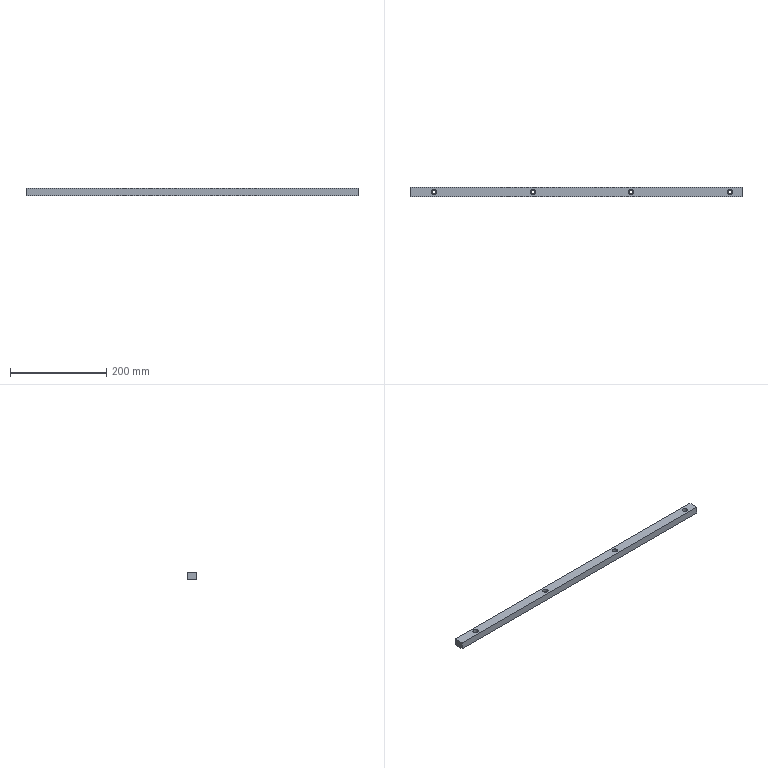Part | SolidWorks | features Extrusion 1, HoleWzd 1, ICE 1 | 1 solid | 26 faces | box 690 x 20 x 15 mm | volume 203293 mm3 | cylinder 16 | plane 10 | commonest cylinder face diameters 6.6 x8 11 x8
STEP:
#1=CARTESIAN_POINT('',(-313.,0.,8.2));
#2=VERTEX_POINT('',#1);
#3=CARTESIAN_POINT('',(-302.,0.,8.2));
#4=VERTEX_POINT('',#3);
#5=CARTESIAN_POINT('',(-307.5,0.,8.2));
#6=DIRECTION('',(0.,0.,1.));
#7=DIRECTION('',(1.,0.,0.));
#8=AXIS2_PLACEMENT_3D('',#5,#6,#7);
#9=CIRCLE('',#8,5.5);
#10=EDGE_CURVE('',#2,#4,#9,.T.);
#11=ORIENTED_EDGE('',*,*,#10,.F.);
#12=CARTESIAN_POINT('',(-313.,0.,15.));
#13=VERTEX_POINT('',#12);
#14=CARTESIAN_POINT('',(-313.,0.,15.));
#15=DIRECTION('',(0.,0.,1.));
#16=VECTOR('',#15,1000.);
#17=LINE('',#14,#16);
#18=EDGE_CURVE('',#2,#13,#17,.T.);
#19=ORIENTED_EDGE('',*,*,#18,.T.);
#20=CARTESIAN_POINT('',(-302.,0.,15.));
#21=VERTEX_POINT('',#20);
#22=CARTESIAN_POINT('',(-307.5,0.,15.));
#23=DIRECTION('',(0.,0.,1.));
#24=DIRECTION('',(1.,0.,0.));
#25=AXIS2_PLACEMENT_3D('',#22,#23,#24);
#26=CIRCLE('',#25,5.5);
#27=EDGE_CURVE('',#13,#21,#26,.T.);
#28=ORIENTED_EDGE('',*,*,#27,.T.);
#29=CARTESIAN_POINT('',(-302.,0.,15.));
#30=DIRECTION('',(0.,0.,1.));
#31=VECTOR('',#30,1000.);
#32=LINE('',#29,#31);
#33=EDGE_CURVE('',#4,#21,#32,.T.);
#34=ORIENTED_EDGE('',*,*,#33,.F.);
#35=EDGE_LOOP('',(#11,#19,#28,#34));
#36=FACE_OUTER_BOUND('',#35,.T.);
#37=CARTESIAN_POINT('',(-307.5,0.,15.));
#38=DIRECTION('',(0.,0.,1.));
#39=DIRECTION('',(1.,0.,0.));
#40=AXIS2_PLACEMENT_3D('',#37,#38,#39);
#41=CYLINDRICAL_SURFACE('',#40,5.5);
#42=ADVANCED_FACE('',(#36),#41,.F.);
#43=CARTESIAN_POINT('',(-310.8,0.,0.));
#44=VERTEX_POINT('',#43);
#45=CARTESIAN_POINT('',(-304.2,0.,0.));
#46=VERTEX_POINT('',#45);
#47=CARTESIAN_POINT('',(-307.5,0.,0.));
#48=DIRECTION('',(0.,0.,1.));
#49=DIRECTION('',(1.,0.,0.));
#50=AXIS2_PLACEMENT_3D('',#47,#48,#49);
#51=CIRCLE('',#50,3.3);
#52=EDGE_CURVE('',#44,#46,#51,.T.);
#53=ORIENTED_EDGE('',*,*,#52,.F.);
#54=CARTESIAN_POINT('',(-310.8,0.,8.2));
#55=VERTEX_POINT('',#54);
#56=CARTESIAN_POINT('',(-310.8,0.,15.));
#57=DIRECTION('',(0.,0.,1.));
#58=VECTOR('',#57,1000.);
#59=LINE('',#56,#58);
#60=EDGE_CURVE('',#44,#55,#59,.T.);
#61=ORIENTED_EDGE('',*,*,#60,.T.);
#62=CARTESIAN_POINT('',(-304.2,0.,8.2));
#63=VERTEX_POINT('',#62);
#64=CARTESIAN_POINT('',(-307.5,0.,8.2));
#65=DIRECTION('',(0.,0.,1.));
#66=DIRECTION('',(1.,0.,0.));
#67=AXIS2_PLACEMENT_3D('',#64,#65,#66);
#68=CIRCLE('',#67,3.3);
#69=EDGE_CURVE('',#55,#63,#68,.T.);
#70=ORIENTED_EDGE('',*,*,#69,.T.);
#71=CARTESIAN_POINT('',(-304.2,0.,15.));
#72=DIRECTION('',(0.,0.,1.));
#73=VECTOR('',#72,1000.);
#74=LINE('',#71,#73);
#75=EDGE_CURVE('',#46,#63,#74,.T.);
#76=ORIENTED_EDGE('',*,*,#75,.F.);
#77=EDGE_LOOP('',(#53,#61,#70,#76));
#78=FACE_OUTER_BOUND('',#77,.T.);
#79=CARTESIAN_POINT('',(-307.5,0.,15.));
#80=DIRECTION('',(0.,0.,1.));
#81=DIRECTION('',(1.,0.,0.));
#82=AXIS2_PLACEMENT_3D('',#79,#80,#81);
#83=CYLINDRICAL_SURFACE('',#82,3.3);
#84=ADVANCED_FACE('',(#78),#83,.F.);
#85=CARTESIAN_POINT('',(302.,0.,8.2));
#86=VERTEX_POINT('',#85);
#87=CARTESIAN_POINT('',(313.,0.,8.2));
#88=VERTEX_POINT('',#87);
#89=CARTESIAN_POINT('',(307.5,0.,8.2));
#90=DIRECTION('',(0.,0.,1.));
#91=DIRECTION('',(1.,0.,0.));
#92=AXIS2_PLACEMENT_3D('',#89,#90,#91);
#93=CIRCLE('',#92,5.5);
#94=EDGE_CURVE('',#86,#88,#93,.T.);
#95=ORIENTED_EDGE('',*,*,#94,.F.);
#96=CARTESIAN_POINT('',(302.,0.,15.));
#97=VERTEX_POINT('',#96);
#98=CARTESIAN_POINT('',(302.,0.,15.));
#99=DIRECTION('',(0.,0.,1.));
#100=VECTOR('',#99,1000.);
#101=LINE('',#98,#100);
#102=EDGE_CURVE('',#86,#97,#101,.T.);
#103=ORIENTED_EDGE('',*,*,#102,.T.);
#104=CARTESIAN_POINT('',(313.,0.,15.));
#105=VERTEX_POINT('',#104);
#106=CARTESIAN_POINT('',(307.5,0.,15.));
#107=DIRECTION('',(0.,0.,1.));
#108=DIRECTION('',(1.,0.,0.));
#109=AXIS2_PLACEMENT_3D('',#106,#107,#108);
#110=CIRCLE('',#109,5.5);
#111=EDGE_CURVE('',#97,#105,#110,.T.);
#112=ORIENTED_EDGE('',*,*,#111,.T.);
#113=CARTESIAN_POINT('',(313.,0.,15.));
#114=DIRECTION('',(0.,0.,1.));
#115=VECTOR('',#114,1000.);
#116=LINE('',#113,#115);
#117=EDGE_CURVE('',#88,#105,#116,.T.);
#118=ORIENTED_EDGE('',*,*,#117,.F.);
#119=EDGE_LOOP('',(#95,#103,#112,#118));
#120=FACE_OUTER_BOUND('',#119,.T.);
#121=CARTESIAN_POINT('',(307.5,0.,15.));
#122=DIRECTION('',(0.,0.,1.));
#123=DIRECTION('',(1.,0.,0.));
#124=AXIS2_PLACEMENT_3D('',#121,#122,#123);
#125=CYLINDRICAL_SURFACE('',#124,5.5);
#126=ADVANCED_FACE('',(#120),#125,.F.);
#127=CARTESIAN_POINT('',(304.2,0.,0.));
#128=VERTEX_POINT('',#127);
#129=CARTESIAN_POINT('',(310.8,0.,0.));
#130=VERTEX_POINT('',#129);
#131=CARTESIAN_POINT('',(307.5,0.,0.));
#132=DIRECTION('',(0.,0.,1.));
#133=DIRECTION('',(1.,0.,0.));
#134=AXIS2_PLACEMENT_3D('',#131,#132,#133);
#135=CIRCLE('',#134,3.3);
#136=EDGE_CURVE('',#128,#130,#135,.T.);
#137=ORIENTED_EDGE('',*,*,#136,.F.);
#138=CARTESIAN_POINT('',(304.2,0.,8.2));
#139=VERTEX_POINT('',#138);
#140=CARTESIAN_POINT('',(304.2,0.,15.));
#141=DIRECTION('',(0.,0.,1.));
#142=VECTOR('',#141,1000.);
#143=LINE('',#140,#142);
#144=EDGE_CURVE('',#128,#139,#143,.T.);
#145=ORIENTED_EDGE('',*,*,#144,.T.);
#146=CARTESIAN_POINT('',(310.8,0.,8.2));
#147=VERTEX_POINT('',#146);
#148=CARTESIAN_POINT('',(307.5,0.,8.2));
#149=DIRECTION('',(0.,0.,1.));
#150=DIRECTION('',(1.,0.,0.));
#151=AXIS2_PLACEMENT_3D('',#148,#149,#150);
#152=CIRCLE('',#151,3.3);
#153=EDGE_CURVE('',#139,#147,#152,.T.);
#154=ORIENTED_EDGE('',*,*,#153,.T.);
#155=CARTESIAN_POINT('',(310.8,0.,15.));
#156=DIRECTION('',(0.,0.,1.));
#157=VECTOR('',#156,1000.);
#158=LINE('',#155,#157);
#159=EDGE_CURVE('',#130,#147,#158,.T.);
#160=ORIENTED_EDGE('',*,*,#159,.F.);
#161=EDGE_LOOP('',(#137,#145,#154,#160));
#162=FACE_OUTER_BOUND('',#161,.T.);
#163=CARTESIAN_POINT('',(307.5,0.,15.));
#164=DIRECTION('',(0.,0.,1.));
#165=DIRECTION('',(1.,0.,0.));
#166=AXIS2_PLACEMENT_3D('',#163,#164,#165);
#167=CYLINDRICAL_SURFACE('',#166,3.3);
#168=ADVANCED_FACE('',(#162),#167,.F.);
#169=CARTESIAN_POINT('',(-108.,0.,8.2));
#170=VERTEX_POINT('',#169);
#171=CARTESIAN_POINT('',(-97.,0.,8.2));
#172=VERTEX_POINT('',#171);
#173=CARTESIAN_POINT('',(-102.5,0.,8.2));
#174=DIRECTION('',(0.,0.,1.));
#175=DIRECTION('',(1.,0.,0.));
#176=AXIS2_PLACEMENT_3D('',#173,#174,#175);
#177=CIRCLE('',#176,5.5);
#178=EDGE_CURVE('',#170,#172,#177,.T.);
#179=ORIENTED_EDGE('',*,*,#178,.F.);
#180=CARTESIAN_POINT('',(-108.,0.,15.));
#181=VERTEX_POINT('',#180);
#182=CARTESIAN_POINT('',(-108.,0.,15.));
#183=DIRECTION('',(0.,0.,1.));
#184=VECTOR('',#183,1000.);
#185=LINE('',#182,#184);
#186=EDGE_CURVE('',#170,#181,#185,.T.);
#187=ORIENTED_EDGE('',*,*,#186,.T.);
#188=CARTESIAN_POINT('',(-97.,0.,15.));
#189=VERTEX_POINT('',#188);
#190=CARTESIAN_POINT('',(-102.5,0.,15.));
#191=DIRECTION('',(0.,0.,1.));
#192=DIRECTION('',(1.,0.,0.));
#193=AXIS2_PLACEMENT_3D('',#190,#191,#192);
#194=CIRCLE('',#193,5.5);
#195=EDGE_CURVE('',#181,#189,#194,.T.);
#196=ORIENTED_EDGE('',*,*,#195,.T.);
#197=CARTESIAN_POINT('',(-97.,0.,15.));
#198=DIRECTION('',(0.,0.,1.));
#199=VECTOR('',#198,1000.);
#200=LINE('',#197,#199);
#201=EDGE_CURVE('',#172,#189,#200,.T.);
#202=ORIENTED_EDGE('',*,*,#201,.F.);
#203=EDGE_LOOP('',(#179,#187,#196,#202));
#204=FACE_OUTER_BOUND('',#203,.T.);
#205=CARTESIAN_POINT('',(-102.5,0.,15.));
#206=DIRECTION('',(0.,0.,1.));
#207=DIRECTION('',(1.,0.,0.));
#208=AXIS2_PLACEMENT_3D('',#205,#206,#207);
#209=CYLINDRICAL_SURFACE('',#208,5.5);
#210=ADVANCED_FACE('',(#204),#209,.F.);
#211=CARTESIAN_POINT('',(-105.8,0.,0.));
#212=VERTEX_POINT('',#211);
#213=CARTESIAN_POINT('',(-99.2,0.,0.));
#214=VERTEX_POINT('',#213);
#215=CARTESIAN_POINT('',(-102.5,0.,0.));
#216=DIRECTION('',(0.,0.,1.));
#217=DIRECTION('',(1.,0.,0.));
#218=AXIS2_PLACEMENT_3D('',#215,#216,#217);
#219=CIRCLE('',#218,3.3);
#220=EDGE_CURVE('',#212,#214,#219,.T.);
#221=ORIENTED_EDGE('',*,*,#220,.F.);
#222=CARTESIAN_POINT('',(-105.8,0.,8.2));
#223=VERTEX_POINT('',#222);
#224=CARTESIAN_POINT('',(-105.8,0.,15.));
#225=DIRECTION('',(0.,0.,1.));
#226=VECTOR('',#225,1000.);
#227=LINE('',#224,#226);
#228=EDGE_CURVE('',#212,#223,#227,.T.);
#229=ORIENTED_EDGE('',*,*,#228,.T.);
#230=CARTESIAN_POINT('',(-99.2,0.,8.2));
#231=VERTEX_POINT('',#230);
#232=CARTESIAN_POINT('',(-102.5,0.,8.2));
#233=DIRECTION('',(0.,0.,1.));
#234=DIRECTION('',(1.,0.,0.));
#235=AXIS2_PLACEMENT_3D('',#232,#233,#234);
#236=CIRCLE('',#235,3.3);
#237=EDGE_CURVE('',#223,#231,#236,.T.);
#238=ORIENTED_EDGE('',*,*,#237,.T.);
#239=CARTESIAN_POINT('',(-99.2,0.,15.));
#240=DIRECTION('',(0.,0.,1.));
#241=VECTOR('',#240,1000.);
#242=LINE('',#239,#241);
#243=EDGE_CURVE('',#214,#231,#242,.T.);
#244=ORIENTED_EDGE('',*,*,#243,.F.);
#245=EDGE_LOOP('',(#221,#229,#238,#244));
#246=FACE_OUTER_BOUND('',#245,.T.);
#247=CARTESIAN_POINT('',(-102.5,0.,15.));
#248=DIRECTION('',(0.,0.,1.));
#249=DIRECTION('',(1.,0.,0.));
#250=AXIS2_PLACEMENT_3D('',#247,#248,#249);
#251=CYLINDRICAL_SURFACE('',#250,3.3);
#252=ADVANCED_FACE('',(#246),#251,.F.);
#253=CARTESIAN_POINT('',(97.,0.,8.2));
#254=VERTEX_POINT('',#253);
#255=CARTESIAN_POINT('',(108.,0.,8.2));
#256=VERTEX_POINT('',#255);
#257=CARTESIAN_POINT('',(102.5,0.,8.2));
#258=DIRECTION('',(0.,0.,1.));
#259=DIRECTION('',(1.,0.,0.));
#260=AXIS2_PLACEMENT_3D('',#257,#258,#259);
#261=CIRCLE('',#260,5.5);
#262=EDGE_CURVE('',#254,#256,#261,.T.);
#263=ORIENTED_EDGE('',*,*,#262,.F.);
#264=CARTESIAN_POINT('',(97.,0.,15.));
#265=VERTEX_POINT('',#264);
#266=CARTESIAN_POINT('',(97.,0.,15.));
#267=DIRECTION('',(0.,0.,1.));
#268=VECTOR('',#267,1000.);
#269=LINE('',#266,#268);
#270=EDGE_CURVE('',#254,#265,#269,.T.);
#271=ORIENTED_EDGE('',*,*,#270,.T.);
#272=CARTESIAN_POINT('',(108.,0.,15.));
#273=VERTEX_POINT('',#272);
#274=CARTESIAN_POINT('',(102.5,0.,15.));
#275=DIRECTION('',(0.,0.,1.));
#276=DIRECTION('',(1.,0.,0.));
#277=AXIS2_PLACEMENT_3D('',#274,#275,#276);
#278=CIRCLE('',#277,5.5);
#279=EDGE_CURVE('',#265,#273,#278,.T.);
#280=ORIENTED_EDGE('',*,*,#279,.T.);
#281=CARTESIAN_POINT('',(108.,0.,15.));
#282=DIRECTION('',(0.,0.,1.));
#283=VECTOR('',#282,1000.);
#284=LINE('',#281,#283);
#285=EDGE_CURVE('',#256,#273,#284,.T.);
#286=ORIENTED_EDGE('',*,*,#285,.F.);
#287=EDGE_LOOP('',(#263,#271,#280,#286));
#288=FACE_OUTER_BOUND('',#287,.T.);
#289=CARTESIAN_POINT('',(102.5,0.,15.));
#290=DIRECTION('',(0.,0.,1.));
#291=DIRECTION('',(1.,0.,0.));
#292=AXIS2_PLACEMENT_3D('',#289,#290,#291);
#293=CYLINDRICAL_SURFACE('',#292,5.5);
#294=ADVANCED_FACE('',(#288),#293,.F.);
#295=CARTESIAN_POINT('',(99.2,0.,0.));
#296=VERTEX_POINT('',#295);
#297=CARTESIAN_POINT('',(105.8,0.,0.));
#298=VERTEX_POINT('',#297);
#299=CARTESIAN_POINT('',(102.5,0.,0.));
#300=DIRECTION('',(0.,0.,1.));
#301=DIRECTION('',(1.,0.,0.));
#302=AXIS2_PLACEMENT_3D('',#299,#300,#301);
#303=CIRCLE('',#302,3.3);
#304=EDGE_CURVE('',#296,#298,#303,.T.);
#305=ORIENTED_EDGE('',*,*,#304,.F.);
#306=CARTESIAN_POINT('',(99.2,0.,8.2));
#307=VERTEX_POINT('',#306);
#308=CARTESIAN_POINT('',(99.2,0.,15.));
#309=DIRECTION('',(0.,0.,1.));
#310=VECTOR('',#309,1000.);
#311=LINE('',#308,#310);
#312=EDGE_CURVE('',#296,#307,#311,.T.);
#313=ORIENTED_EDGE('',*,*,#312,.T.);
#314=CARTESIAN_POINT('',(105.8,0.,8.2));
#315=VERTEX_POINT('',#314);
#316=CARTESIAN_POINT('',(102.5,0.,8.2));
#317=DIRECTION('',(0.,0.,1.));
#318=DIRECTION('',(1.,0.,0.));
#319=AXIS2_PLACEMENT_3D('',#316,#317,#318);
#320=CIRCLE('',#319,3.3);
#321=EDGE_CURVE('',#307,#315,#320,.T.);
#322=ORIENTED_EDGE('',*,*,#321,.T.);
#323=CARTESIAN_POINT('',(105.8,0.,15.));
#324=DIRECTION('',(0.,0.,1.));
#325=VECTOR('',#324,1000.);
#326=LINE('',#323,#325);
#327=EDGE_CURVE('',#298,#315,#326,.T.);
#328=ORIENTED_EDGE('',*,*,#327,.F.);
#329=EDGE_LOOP('',(#305,#313,#322,#328));
#330=FACE_OUTER_BOUND('',#329,.T.);
#331=CARTESIAN_POINT('',(102.5,0.,15.));
#332=DIRECTION('',(0.,0.,1.));
#333=DIRECTION('',(1.,0.,0.));
#334=AXIS2_PLACEMENT_3D('',#331,#332,#333);
#335=CYLINDRICAL_SURFACE('',#334,3.3);
#336=ADVANCED_FACE('',(#330),#335,.F.);
#337=CARTESIAN_POINT('',(332.5,-10.,0.));
#338=VERTEX_POINT('',#337);
#339=CARTESIAN_POINT('',(332.5,10.,0.));
#340=VERTEX_POINT('',#339);
#341=CARTESIAN_POINT('',(332.5,10.,0.));
#342=DIRECTION('',(0.,1.,0.));
#343=VECTOR('',#342,1000.);
#344=LINE('',#341,#343);
#345=EDGE_CURVE('',#338,#340,#344,.T.);
#346=ORIENTED_EDGE('',*,*,#345,.T.);
#347=CARTESIAN_POINT('',(332.5,10.,15.));
#348=VERTEX_POINT('',#347);
#349=CARTESIAN_POINT('',(332.5,10.,15.));
#350=DIRECTION('',(0.,0.,-1.));
#351=VECTOR('',#350,1000.);
#352=LINE('',#349,#351);
#353=EDGE_CURVE('',#348,#340,#352,.T.);
#354=ORIENTED_EDGE('',*,*,#353,.F.);
#355=CARTESIAN_POINT('',(332.5,-10.,15.));
#356=VERTEX_POINT('',#355);
#357=CARTESIAN_POINT('',(332.5,10.,15.));
#358=DIRECTION('',(0.,1.,0.));
#359=VECTOR('',#358,1000.);
#360=LINE('',#357,#359);
#361=EDGE_CURVE('',#356,#348,#360,.T.);
#362=ORIENTED_EDGE('',*,*,#361,.F.);
#363=CARTESIAN_POINT('',(332.5,-10.,15.));
#364=DIRECTION('',(0.,0.,-1.));
#365=VECTOR('',#364,1000.);
#366=LINE('',#363,#365);
#367=EDGE_CURVE('',#356,#338,#366,.T.);
#368=ORIENTED_EDGE('',*,*,#367,.T.);
#369=EDGE_LOOP('',(#346,#354,#362,#368));
#370=FACE_OUTER_BOUND('',#369,.T.);
#371=CARTESIAN_POINT('',(332.5,10.,15.));
#372=DIRECTION('',(-1.,0.,0.));
#373=DIRECTION('',(0.,0.,1.));
#374=AXIS2_PLACEMENT_3D('',#371,#372,#373);
#375=PLANE('',#374);
#376=ADVANCED_FACE('',(#370),#375,.F.);
#377=CARTESIAN_POINT('',(-357.5,10.,0.));
#378=VERTEX_POINT('',#377);
#379=CARTESIAN_POINT('',(-332.5,10.,0.));
#380=DIRECTION('',(-1.,0.,0.));
#381=VECTOR('',#380,1000.);
#382=LINE('',#379,#381);
#383=EDGE_CURVE('',#340,#378,#382,.T.);
#384=ORIENTED_EDGE('',*,*,#383,.T.);
#385=CARTESIAN_POINT('',(-357.5,10.,15.));
#386=VERTEX_POINT('',#385);
#387=CARTESIAN_POINT('',(-357.5,10.,15.));
#388=DIRECTION('',(0.,0.,-1.));
#389=VECTOR('',#388,1000.);
#390=LINE('',#387,#389);
#391=EDGE_CURVE('',#386,#378,#390,.T.);
#392=ORIENTED_EDGE('',*,*,#391,.F.);
#393=CARTESIAN_POINT('',(-332.5,10.,15.));
#394=DIRECTION('',(-1.,0.,0.));
#395=VECTOR('',#394,1000.);
#396=LINE('',#393,#395);
#397=EDGE_CURVE('',#348,#386,#396,.T.);
#398=ORIENTED_EDGE('',*,*,#397,.F.);
#399=ORIENTED_EDGE('',*,*,#353,.T.);
#400=EDGE_LOOP('',(#384,#392,#398,#399));
#401=FACE_OUTER_BOUND('',#400,.T.);
#402=CARTESIAN_POINT('',(-332.5,10.,15.));
#403=DIRECTION('',(0.,-1.,0.));
#404=DIRECTION('',(0.,0.,-1.));
#405=AXIS2_PLACEMENT_3D('',#402,#403,#404);
#406=PLANE('',#405);
#407=ADVANCED_FACE('',(#401),#406,.F.);
#408=CARTESIAN_POINT('',(-357.5,-10.,0.));
#409=VERTEX_POINT('',#408);
#410=CARTESIAN_POINT('',(-332.5,-10.,0.));
#411=DIRECTION('',(1.,0.,0.));
#412=VECTOR('',#411,1000.);
#413=LINE('',#410,#412);
#414=EDGE_CURVE('',#409,#338,#413,.T.);
#415=ORIENTED_EDGE('',*,*,#414,.T.);
#416=ORIENTED_EDGE('',*,*,#367,.F.);
#417=CARTESIAN_POINT('',(-357.5,-10.,15.));
#418=VERTEX_POINT('',#417);
#419=CARTESIAN_POINT('',(-332.5,-10.,15.));
#420=DIRECTION('',(1.,0.,0.));
#421=VECTOR('',#420,1000.);
#422=LINE('',#419,#421);
#423=EDGE_CURVE('',#418,#356,#422,.T.);
#424=ORIENTED_EDGE('',*,*,#423,.F.);
#425=CARTESIAN_POINT('',(-357.5,-10.,0.));
#426=DIRECTION('',(0.,0.,1.));
#427=VECTOR('',#426,1000.);
#428=LINE('',#425,#427);
#429=EDGE_CURVE('',#409,#418,#428,.T.);
#430=ORIENTED_EDGE('',*,*,#429,.F.);
#431=EDGE_LOOP('',(#415,#416,#424,#430));
#432=FACE_OUTER_BOUND('',#431,.T.);
#433=CARTESIAN_POINT('',(-332.5,-10.,15.));
#434=DIRECTION('',(0.,1.,0.));
#435=DIRECTION('',(0.,0.,1.));
#436=AXIS2_PLACEMENT_3D('',#433,#434,#435);
#437=PLANE('',#436);
#438=ADVANCED_FACE('',(#432),#437,.F.);
#439=CARTESIAN_POINT('',(-307.5,0.,15.));
#440=DIRECTION('',(0.,0.,1.));
#441=DIRECTION('',(1.,0.,0.));
#442=AXIS2_PLACEMENT_3D('',#439,#440,#441);
#443=CIRCLE('',#442,5.5);
#444=EDGE_CURVE('',#21,#13,#443,.T.);
#445=ORIENTED_EDGE('',*,*,#444,.F.);
#446=ORIENTED_EDGE('',*,*,#27,.F.);
#447=EDGE_LOOP('',(#445,#446));
#448=FACE_BOUND('',#447,.T.);
#449=CARTESIAN_POINT('',(307.5,0.,15.));
#450=DIRECTION('',(0.,0.,1.));
#451=DIRECTION('',(1.,0.,0.));
#452=AXIS2_PLACEMENT_3D('',#449,#450,#451);
#453=CIRCLE('',#452,5.5);
#454=EDGE_CURVE('',#105,#97,#453,.T.);
#455=ORIENTED_EDGE('',*,*,#454,.F.);
#456=ORIENTED_EDGE('',*,*,#111,.F.);
#457=EDGE_LOOP('',(#455,#456));
#458=FACE_BOUND('',#457,.T.);
#459=CARTESIAN_POINT('',(-102.5,0.,15.));
#460=DIRECTION('',(0.,0.,1.));
#461=DIRECTION('',(1.,0.,0.));
#462=AXIS2_PLACEMENT_3D('',#459,#460,#461);
#463=CIRCLE('',#462,5.5);
#464=EDGE_CURVE('',#189,#181,#463,.T.);
#465=ORIENTED_EDGE('',*,*,#464,.F.);
#466=ORIENTED_EDGE('',*,*,#195,.F.);
#467=EDGE_LOOP('',(#465,#466));
#468=FACE_BOUND('',#467,.T.);
#469=CARTESIAN_POINT('',(102.5,0.,15.));
#470=DIRECTION('',(0.,0.,1.));
#471=DIRECTION('',(1.,0.,0.));
#472=AXIS2_PLACEMENT_3D('',#469,#470,#471);
#473=CIRCLE('',#472,5.5);
#474=EDGE_CURVE('',#273,#265,#473,.T.);
#475=ORIENTED_EDGE('',*,*,#474,.F.);
#476=ORIENTED_EDGE('',*,*,#279,.F.);
#477=EDGE_LOOP('',(#475,#476));
#478=FACE_BOUND('',#477,.T.);
#479=ORIENTED_EDGE('',*,*,#361,.T.);
#480=ORIENTED_EDGE('',*,*,#397,.T.);
#481=CARTESIAN_POINT('',(-357.5,-10.,15.));
#482=DIRECTION('',(0.,1.,0.));
#483=VECTOR('',#482,1000.);
#484=LINE('',#481,#483);
#485=EDGE_CURVE('',#418,#386,#484,.T.);
#486=ORIENTED_EDGE('',*,*,#485,.F.);
#487=ORIENTED_EDGE('',*,*,#423,.T.);
#488=EDGE_LOOP('',(#479,#480,#486,#487));
#489=FACE_OUTER_BOUND('',#488,.T.);
#490=CARTESIAN_POINT('',(0.,0.,15.));
#491=DIRECTION('',(0.,0.,1.));
#492=DIRECTION('',(1.,0.,0.));
#493=AXIS2_PLACEMENT_3D('',#490,#491,#492);
#494=PLANE('',#493);
#495=ADVANCED_FACE('',(#448,#458,#468,#478,#489),#494,.T.);
#496=CARTESIAN_POINT('',(-307.5,0.,0.));
#497=DIRECTION('',(0.,0.,1.));
#498=DIRECTION('',(1.,0.,0.));
#499=AXIS2_PLACEMENT_3D('',#496,#497,#498);
#500=CIRCLE('',#499,3.3);
#501=EDGE_CURVE('',#46,#44,#500,.T.);
#502=ORIENTED_EDGE('',*,*,#501,.T.);
#503=ORIENTED_EDGE('',*,*,#52,.T.);
#504=EDGE_LOOP('',(#502,#503));
#505=FACE_BOUND('',#504,.T.);
#506=CARTESIAN_POINT('',(307.5,0.,0.));
#507=DIRECTION('',(0.,0.,1.));
#508=DIRECTION('',(1.,0.,0.));
#509=AXIS2_PLACEMENT_3D('',#506,#507,#508);
#510=CIRCLE('',#509,3.3);
#511=EDGE_CURVE('',#130,#128,#510,.T.);
#512=ORIENTED_EDGE('',*,*,#511,.T.);
#513=ORIENTED_EDGE('',*,*,#136,.T.);
#514=EDGE_LOOP('',(#512,#513));
#515=FACE_BOUND('',#514,.T.);
#516=CARTESIAN_POINT('',(-102.5,0.,0.));
#517=DIRECTION('',(0.,0.,1.));
#518=DIRECTION('',(1.,0.,0.));
#519=AXIS2_PLACEMENT_3D('',#516,#517,#518);
#520=CIRCLE('',#519,3.3);
#521=EDGE_CURVE('',#214,#212,#520,.T.);
#522=ORIENTED_EDGE('',*,*,#521,.T.);
#523=ORIENTED_EDGE('',*,*,#220,.T.);
#524=EDGE_LOOP('',(#522,#523));
#525=FACE_BOUND('',#524,.T.);
#526=CARTESIAN_POINT('',(102.5,0.,0.));
#527=DIRECTION('',(0.,0.,1.));
#528=DIRECTION('',(1.,0.,0.));
#529=AXIS2_PLACEMENT_3D('',#526,#527,#528);
#530=CIRCLE('',#529,3.3);
#531=EDGE_CURVE('',#298,#296,#530,.T.);
#532=ORIENTED_EDGE('',*,*,#531,.T.);
#533=ORIENTED_EDGE('',*,*,#304,.T.);
#534=EDGE_LOOP('',(#532,#533));
#535=FACE_BOUND('',#534,.T.);
#536=ORIENTED_EDGE('',*,*,#345,.F.);
#537=ORIENTED_EDGE('',*,*,#414,.F.);
#538=CARTESIAN_POINT('',(-357.5,10.,0.));
#539=DIRECTION('',(0.,-1.,0.));
#540=VECTOR('',#539,1000.);
#541=LINE('',#538,#540);
#542=EDGE_CURVE('',#378,#409,#541,.T.);
#543=ORIENTED_EDGE('',*,*,#542,.F.);
#544=ORIENTED_EDGE('',*,*,#383,.F.);
#545=EDGE_LOOP('',(#536,#537,#543,#544));
#546=FACE_OUTER_BOUND('',#545,.T.);
#547=CARTESIAN_POINT('',(0.,0.,0.));
#548=DIRECTION('',(0.,0.,1.));
#549=DIRECTION('',(1.,0.,0.));
#550=AXIS2_PLACEMENT_3D('',#547,#548,#549);
#551=PLANE('',#550);
#552=ADVANCED_FACE('',(#505,#515,#525,#535,#546),#551,.F.);
#553=ORIENTED_EDGE('',*,*,#312,.F.);
#554=ORIENTED_EDGE('',*,*,#531,.F.);
#555=ORIENTED_EDGE('',*,*,#327,.T.);
#556=CARTESIAN_POINT('',(102.5,0.,8.2));
#557=DIRECTION('',(0.,0.,1.));
#558=DIRECTION('',(1.,0.,0.));
#559=AXIS2_PLACEMENT_3D('',#556,#557,#558);
#560=CIRCLE('',#559,3.3);
#561=EDGE_CURVE('',#315,#307,#560,.T.);
#562=ORIENTED_EDGE('',*,*,#561,.T.);
#563=EDGE_LOOP('',(#553,#554,#555,#562));
#564=FACE_OUTER_BOUND('',#563,.T.);
#565=CARTESIAN_POINT('',(102.5,0.,15.));
#566=DIRECTION('',(0.,0.,1.));
#567=DIRECTION('',(1.,0.,0.));
#568=AXIS2_PLACEMENT_3D('',#565,#566,#567);
#569=CYLINDRICAL_SURFACE('',#568,3.3);
#570=ADVANCED_FACE('',(#564),#569,.F.);
#571=ORIENTED_EDGE('',*,*,#561,.F.);
#572=ORIENTED_EDGE('',*,*,#321,.F.);
#573=EDGE_LOOP('',(#571,#572));
#574=FACE_BOUND('',#573,.T.);
#575=CARTESIAN_POINT('',(102.5,0.,8.2));
#576=DIRECTION('',(0.,0.,1.));
#577=DIRECTION('',(1.,0.,0.));
#578=AXIS2_PLACEMENT_3D('',#575,#576,#577);
#579=CIRCLE('',#578,5.5);
#580=EDGE_CURVE('',#256,#254,#579,.T.);
#581=ORIENTED_EDGE('',*,*,#580,.T.);
#582=ORIENTED_EDGE('',*,*,#262,.T.);
#583=EDGE_LOOP('',(#581,#582));
#584=FACE_OUTER_BOUND('',#583,.T.);
#585=CARTESIAN_POINT('',(105.8,0.,8.2));
#586=DIRECTION('',(0.,0.,-1.));
#587=DIRECTION('',(-1.,0.,0.));
#588=AXIS2_PLACEMENT_3D('',#585,#586,#587);
#589=PLANE('',#588);
#590=ADVANCED_FACE('',(#574,#584),#589,.F.);
#591=ORIENTED_EDGE('',*,*,#270,.F.);
#592=ORIENTED_EDGE('',*,*,#580,.F.);
#593=ORIENTED_EDGE('',*,*,#285,.T.);
#594=ORIENTED_EDGE('',*,*,#474,.T.);
#595=EDGE_LOOP('',(#591,#592,#593,#594));
#596=FACE_OUTER_BOUND('',#595,.T.);
#597=CARTESIAN_POINT('',(102.5,0.,15.));
#598=DIRECTION('',(0.,0.,1.));
#599=DIRECTION('',(1.,0.,0.));
#600=AXIS2_PLACEMENT_3D('',#597,#598,#599);
#601=CYLINDRICAL_SURFACE('',#600,5.5);
#602=ADVANCED_FACE('',(#596),#601,.F.);
#603=ORIENTED_EDGE('',*,*,#228,.F.);
#604=ORIENTED_EDGE('',*,*,#521,.F.);
#605=ORIENTED_EDGE('',*,*,#243,.T.);
#606=CARTESIAN_POINT('',(-102.5,0.,8.2));
#607=DIRECTION('',(0.,0.,1.));
#608=DIRECTION('',(1.,0.,0.));
#609=AXIS2_PLACEMENT_3D('',#606,#607,#608);
#610=CIRCLE('',#609,3.3);
#611=EDGE_CURVE('',#231,#223,#610,.T.);
#612=ORIENTED_EDGE('',*,*,#611,.T.);
#613=EDGE_LOOP('',(#603,#604,#605,#612));
#614=FACE_OUTER_BOUND('',#613,.T.);
#615=CARTESIAN_POINT('',(-102.5,0.,15.));
#616=DIRECTION('',(0.,0.,1.));
#617=DIRECTION('',(1.,0.,0.));
#618=AXIS2_PLACEMENT_3D('',#615,#616,#617);
#619=CYLINDRICAL_SURFACE('',#618,3.3);
#620=ADVANCED_FACE('',(#614),#619,.F.);
#621=ORIENTED_EDGE('',*,*,#611,.F.);
#622=ORIENTED_EDGE('',*,*,#237,.F.);
#623=EDGE_LOOP('',(#621,#622));
#624=FACE_BOUND('',#623,.T.);
#625=CARTESIAN_POINT('',(-102.5,0.,8.2));
#626=DIRECTION('',(0.,0.,1.));
#627=DIRECTION('',(1.,0.,0.));
#628=AXIS2_PLACEMENT_3D('',#625,#626,#627);
#629=CIRCLE('',#628,5.5);
#630=EDGE_CURVE('',#172,#170,#629,.T.);
#631=ORIENTED_EDGE('',*,*,#630,.T.);
#632=ORIENTED_EDGE('',*,*,#178,.T.);
#633=EDGE_LOOP('',(#631,#632));
#634=FACE_OUTER_BOUND('',#633,.T.);
#635=CARTESIAN_POINT('',(-99.2,0.,8.2));
#636=DIRECTION('',(0.,0.,-1.));
#637=DIRECTION('',(-1.,0.,0.));
#638=AXIS2_PLACEMENT_3D('',#635,#636,#637);
#639=PLANE('',#638);
#640=ADVANCED_FACE('',(#624,#634),#639,.F.);
#641=ORIENTED_EDGE('',*,*,#186,.F.);
#642=ORIENTED_EDGE('',*,*,#630,.F.);
#643=ORIENTED_EDGE('',*,*,#201,.T.);
#644=ORIENTED_EDGE('',*,*,#464,.T.);
#645=EDGE_LOOP('',(#641,#642,#643,#644));
#646=FACE_OUTER_BOUND('',#645,.T.);
#647=CARTESIAN_POINT('',(-102.5,0.,15.));
#648=DIRECTION('',(0.,0.,1.));
#649=DIRECTION('',(1.,0.,0.));
#650=AXIS2_PLACEMENT_3D('',#647,#648,#649);
#651=CYLINDRICAL_SURFACE('',#650,5.5);
#652=ADVANCED_FACE('',(#646),#651,.F.);
#653=ORIENTED_EDGE('',*,*,#144,.F.);
#654=ORIENTED_EDGE('',*,*,#511,.F.);
#655=ORIENTED_EDGE('',*,*,#159,.T.);
#656=CARTESIAN_POINT('',(307.5,0.,8.2));
#657=DIRECTION('',(0.,0.,1.));
#658=DIRECTION('',(1.,0.,0.));
#659=AXIS2_PLACEMENT_3D('',#656,#657,#658);
#660=CIRCLE('',#659,3.3);
#661=EDGE_CURVE('',#147,#139,#660,.T.);
#662=ORIENTED_EDGE('',*,*,#661,.T.);
#663=EDGE_LOOP('',(#653,#654,#655,#662));
#664=FACE_OUTER_BOUND('',#663,.T.);
#665=CARTESIAN_POINT('',(307.5,0.,15.));
#666=DIRECTION('',(0.,0.,1.));
#667=DIRECTION('',(1.,0.,0.));
#668=AXIS2_PLACEMENT_3D('',#665,#666,#667);
#669=CYLINDRICAL_SURFACE('',#668,3.3);
#670=ADVANCED_FACE('',(#664),#669,.F.);
#671=ORIENTED_EDGE('',*,*,#661,.F.);
#672=ORIENTED_EDGE('',*,*,#153,.F.);
#673=EDGE_LOOP('',(#671,#672));
#674=FACE_BOUND('',#673,.T.);
#675=CARTESIAN_POINT('',(307.5,0.,8.2));
#676=DIRECTION('',(0.,0.,1.));
#677=DIRECTION('',(1.,0.,0.));
#678=AXIS2_PLACEMENT_3D('',#675,#676,#677);
#679=CIRCLE('',#678,5.5);
#680=EDGE_CURVE('',#88,#86,#679,.T.);
#681=ORIENTED_EDGE('',*,*,#680,.T.);
#682=ORIENTED_EDGE('',*,*,#94,.T.);
#683=EDGE_LOOP('',(#681,#682));
#684=FACE_OUTER_BOUND('',#683,.T.);
#685=CARTESIAN_POINT('',(310.8,0.,8.2));
#686=DIRECTION('',(0.,0.,-1.));
#687=DIRECTION('',(-1.,0.,0.));
#688=AXIS2_PLACEMENT_3D('',#685,#686,#687);
#689=PLANE('',#688);
#690=ADVANCED_FACE('',(#674,#684),#689,.F.);
#691=ORIENTED_EDGE('',*,*,#102,.F.);
#692=ORIENTED_EDGE('',*,*,#680,.F.);
#693=ORIENTED_EDGE('',*,*,#117,.T.);
#694=ORIENTED_EDGE('',*,*,#454,.T.);
#695=EDGE_LOOP('',(#691,#692,#693,#694));
#696=FACE_OUTER_BOUND('',#695,.T.);
#697=CARTESIAN_POINT('',(307.5,0.,15.));
#698=DIRECTION('',(0.,0.,1.));
#699=DIRECTION('',(1.,0.,0.));
#700=AXIS2_PLACEMENT_3D('',#697,#698,#699);
#701=CYLINDRICAL_SURFACE('',#700,5.5);
#702=ADVANCED_FACE('',(#696),#701,.F.);
#703=ORIENTED_EDGE('',*,*,#60,.F.);
#704=ORIENTED_EDGE('',*,*,#501,.F.);
#705=ORIENTED_EDGE('',*,*,#75,.T.);
#706=CARTESIAN_POINT('',(-307.5,0.,8.2));
#707=DIRECTION('',(0.,0.,1.));
#708=DIRECTION('',(1.,0.,0.));
#709=AXIS2_PLACEMENT_3D('',#706,#707,#708);
#710=CIRCLE('',#709,3.3);
#711=EDGE_CURVE('',#63,#55,#710,.T.);
#712=ORIENTED_EDGE('',*,*,#711,.T.);
#713=EDGE_LOOP('',(#703,#704,#705,#712));
#714=FACE_OUTER_BOUND('',#713,.T.);
#715=CARTESIAN_POINT('',(-307.5,0.,15.));
#716=DIRECTION('',(0.,0.,1.));
#717=DIRECTION('',(1.,0.,0.));
#718=AXIS2_PLACEMENT_3D('',#715,#716,#717);
#719=CYLINDRICAL_SURFACE('',#718,3.3);
#720=ADVANCED_FACE('',(#714),#719,.F.);
#721=ORIENTED_EDGE('',*,*,#711,.F.);
#722=ORIENTED_EDGE('',*,*,#69,.F.);
#723=EDGE_LOOP('',(#721,#722));
#724=FACE_BOUND('',#723,.T.);
#725=CARTESIAN_POINT('',(-307.5,0.,8.2));
#726=DIRECTION('',(0.,0.,1.));
#727=DIRECTION('',(1.,0.,0.));
#728=AXIS2_PLACEMENT_3D('',#725,#726,#727);
#729=CIRCLE('',#728,5.5);
#730=EDGE_CURVE('',#4,#2,#729,.T.);
#731=ORIENTED_EDGE('',*,*,#730,.T.);
#732=ORIENTED_EDGE('',*,*,#10,.T.);
#733=EDGE_LOOP('',(#731,#732));
#734=FACE_OUTER_BOUND('',#733,.T.);
#735=CARTESIAN_POINT('',(-304.2,0.,8.2));
#736=DIRECTION('',(0.,0.,-1.));
#737=DIRECTION('',(-1.,0.,0.));
#738=AXIS2_PLACEMENT_3D('',#735,#736,#737);
#739=PLANE('',#738);
#740=ADVANCED_FACE('',(#724,#734),#739,.F.);
#741=ORIENTED_EDGE('',*,*,#18,.F.);
#742=ORIENTED_EDGE('',*,*,#730,.F.);
#743=ORIENTED_EDGE('',*,*,#33,.T.);
#744=ORIENTED_EDGE('',*,*,#444,.T.);
#745=EDGE_LOOP('',(#741,#742,#743,#744));
#746=FACE_OUTER_BOUND('',#745,.T.);
#747=CARTESIAN_POINT('',(-307.5,0.,15.));
#748=DIRECTION('',(0.,0.,1.));
#749=DIRECTION('',(1.,0.,0.));
#750=AXIS2_PLACEMENT_3D('',#747,#748,#749);
#751=CYLINDRICAL_SURFACE('',#750,5.5);
#752=ADVANCED_FACE('',(#746),#751,.F.);
#753=ORIENTED_EDGE('',*,*,#391,.T.);
#754=ORIENTED_EDGE('',*,*,#542,.T.);
#755=ORIENTED_EDGE('',*,*,#429,.T.);
#756=ORIENTED_EDGE('',*,*,#485,.T.);
#757=EDGE_LOOP('',(#753,#754,#755,#756));
#758=FACE_OUTER_BOUND('',#757,.T.);
#759=CARTESIAN_POINT('',(-357.5,0.,0.));
#760=DIRECTION('',(-1.,0.,0.));
#761=DIRECTION('',(0.,0.,1.));
#762=AXIS2_PLACEMENT_3D('',#759,#760,#761);
#763=PLANE('',#762);
#764=ADVANCED_FACE('',(#758),#763,.T.);
#765=CLOSED_SHELL('',(#42,#84,#126,#168,#210,#252,#294,#336,#376,#407,#438,#495,#552,#570,#590,#602,#620,#640,#652,#670,#690,#702,#720,#740,#752,#764));
#766=MANIFOLD_SOLID_BREP('',#765);
#767=CARTESIAN_POINT('',(0.,0.,0.));
#768=DIRECTION('',(0.,0.,1.));
#769=DIRECTION('',(1.,0.,0.));
#770=AXIS2_PLACEMENT_3D('',#767,#768,#769);
#771=(LENGTH_UNIT()NAMED_UNIT(*)SI_UNIT(.MILLI.,.METRE.));
#772=UNCERTAINTY_MEASURE_WITH_UNIT(LENGTH_MEASURE(0.00001),#771,'','');
#773=(NAMED_UNIT(*)PLANE_ANGLE_UNIT()SI_UNIT($,.RADIAN.));
#774=(NAMED_UNIT(*)SI_UNIT($,.STERADIAN.)SOLID_ANGLE_UNIT());
#775=(GEOMETRIC_REPRESENTATION_CONTEXT(3)GLOBAL_UNCERTAINTY_ASSIGNED_CONTEXT((#772))GLOBAL_UNIT_ASSIGNED_CONTEXT((#771,#773,#774))REPRESENTATION_CONTEXT('',''));
#776=ADVANCED_BREP_SHAPE_REPRESENTATION('',(#766,#770),#775);